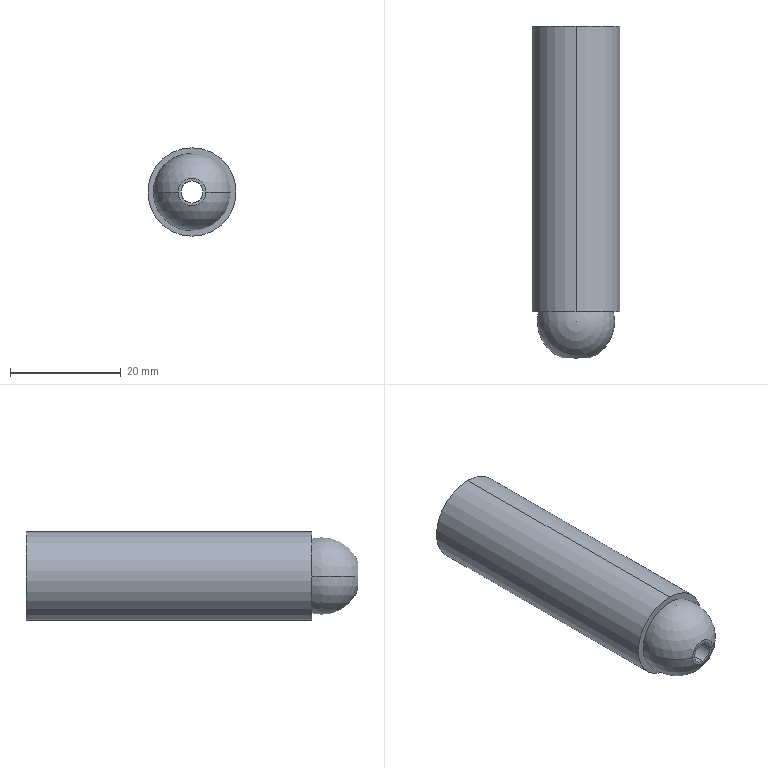Part | SolidWorks | features Revolution 1 | 1 solid | 11 faces | box 16 x 60 x 16 mm | volume 9983 mm3 | cylinder 4 | sphere 4 | plane 3 | commonest cylinder face diameters 4 x2 16 x2
STEP:
#1=CARTESIAN_POINT('',(0.,60.,-8.));
#2=VERTEX_POINT('',#1);
#3=CARTESIAN_POINT('',(0.,60.,8.));
#4=VERTEX_POINT('',#3);
#5=CARTESIAN_POINT('',(0.,60.,0.));
#6=DIRECTION('',(0.,-1.,0.));
#7=DIRECTION('',(0.,0.,-1.));
#8=AXIS2_PLACEMENT_3D('',#5,#6,#7);
#9=CIRCLE('',#8,8.);
#10=EDGE_CURVE('',#2,#4,#9,.T.);
#11=ORIENTED_EDGE('',*,*,#10,.T.);
#12=CARTESIAN_POINT('',(0.,8.392,8.));
#13=VERTEX_POINT('',#12);
#14=CARTESIAN_POINT('',(0.,0.,8.));
#15=DIRECTION('',(0.,-1.,0.));
#16=VECTOR('',#15,1000.);
#17=LINE('',#14,#16);
#18=EDGE_CURVE('',#4,#13,#17,.T.);
#19=ORIENTED_EDGE('',*,*,#18,.T.);
#20=CARTESIAN_POINT('',(0.,8.392,-8.));
#21=VERTEX_POINT('',#20);
#22=CARTESIAN_POINT('',(0.,8.392,0.));
#23=DIRECTION('',(0.,-1.,0.));
#24=DIRECTION('',(0.,0.,-1.));
#25=AXIS2_PLACEMENT_3D('',#22,#23,#24);
#26=CIRCLE('',#25,8.);
#27=EDGE_CURVE('',#21,#13,#26,.T.);
#28=ORIENTED_EDGE('',*,*,#27,.F.);
#29=CARTESIAN_POINT('',(0.,0.,-8.));
#30=DIRECTION('',(0.,-1.,0.));
#31=VECTOR('',#30,1000.);
#32=LINE('',#29,#31);
#33=EDGE_CURVE('',#2,#21,#32,.T.);
#34=ORIENTED_EDGE('',*,*,#33,.F.);
#35=EDGE_LOOP('',(#11,#19,#28,#34));
#36=FACE_OUTER_BOUND('',#35,.T.);
#37=CARTESIAN_POINT('',(0.,0.,0.));
#38=DIRECTION('',(0.,-1.,0.));
#39=DIRECTION('',(0.,0.,-1.));
#40=AXIS2_PLACEMENT_3D('',#37,#38,#39);
#41=CYLINDRICAL_SURFACE('',#40,8.);
#42=ADVANCED_FACE('',(#36),#41,.T.);
#43=CARTESIAN_POINT('',(7.,60.,0.));
#44=VERTEX_POINT('',#43);
#45=CARTESIAN_POINT('',(-7.,60.,0.));
#46=VERTEX_POINT('',#45);
#47=CARTESIAN_POINT('',(0.,60.,0.));
#48=DIRECTION('',(0.,-1.,0.));
#49=DIRECTION('',(0.,0.,-1.));
#50=AXIS2_PLACEMENT_3D('',#47,#48,#49);
#51=CIRCLE('',#50,7.);
#52=EDGE_CURVE('',#44,#46,#51,.T.);
#53=ORIENTED_EDGE('',*,*,#52,.F.);
#54=CARTESIAN_POINT('',(2.,53.292,0.));
#55=VERTEX_POINT('',#54);
#56=CARTESIAN_POINT('',(0.,60.,0.));
#57=DIRECTION('',(0.,0.,-1.));
#58=DIRECTION('',(-1.,0.,0.));
#59=AXIS2_PLACEMENT_3D('',#56,#57,#58);
#60=CIRCLE('',#59,7.);
#61=EDGE_CURVE('',#44,#55,#60,.T.);
#62=ORIENTED_EDGE('',*,*,#61,.T.);
#63=CARTESIAN_POINT('',(0.,53.292,2.));
#64=VERTEX_POINT('',#63);
#65=CARTESIAN_POINT('',(0.,53.292,0.));
#66=DIRECTION('',(0.,-1.,0.));
#67=DIRECTION('',(0.,0.,-1.));
#68=AXIS2_PLACEMENT_3D('',#65,#66,#67);
#69=CIRCLE('',#68,2.);
#70=EDGE_CURVE('',#55,#64,#69,.T.);
#71=ORIENTED_EDGE('',*,*,#70,.T.);
#72=CARTESIAN_POINT('',(-2.,53.292,0.));
#73=VERTEX_POINT('',#72);
#74=CARTESIAN_POINT('',(0.,53.292,0.));
#75=DIRECTION('',(0.,-1.,0.));
#76=DIRECTION('',(0.,0.,-1.));
#77=AXIS2_PLACEMENT_3D('',#74,#75,#76);
#78=CIRCLE('',#77,2.);
#79=EDGE_CURVE('',#64,#73,#78,.T.);
#80=ORIENTED_EDGE('',*,*,#79,.T.);
#81=CARTESIAN_POINT('',(0.,60.,0.));
#82=DIRECTION('',(0.,0.,1.));
#83=DIRECTION('',(1.,0.,0.));
#84=AXIS2_PLACEMENT_3D('',#81,#82,#83);
#85=CIRCLE('',#84,7.);
#86=EDGE_CURVE('',#46,#73,#85,.T.);
#87=ORIENTED_EDGE('',*,*,#86,.F.);
#88=EDGE_LOOP('',(#53,#62,#71,#80,#87));
#89=FACE_OUTER_BOUND('',#88,.T.);
#90=CARTESIAN_POINT('',(0.,60.,0.));
#91=DIRECTION('',(0.,0.,-1.));
#92=DIRECTION('',(-1.,0.,0.));
#93=AXIS2_PLACEMENT_3D('',#90,#91,#92);
#94=SPHERICAL_SURFACE('',#93,7.);
#95=ADVANCED_FACE('',(#89),#94,.F.);
#96=ORIENTED_EDGE('',*,*,#79,.F.);
#97=CARTESIAN_POINT('',(0.,0.,2.));
#98=VERTEX_POINT('',#97);
#99=CARTESIAN_POINT('',(0.,0.,2.));
#100=DIRECTION('',(0.,-1.,0.));
#101=VECTOR('',#100,1000.);
#102=LINE('',#99,#101);
#103=EDGE_CURVE('',#64,#98,#102,.T.);
#104=ORIENTED_EDGE('',*,*,#103,.T.);
#105=CARTESIAN_POINT('',(0.,0.,-2.));
#106=VERTEX_POINT('',#105);
#107=CARTESIAN_POINT('',(0.,0.,0.));
#108=DIRECTION('',(0.,-1.,0.));
#109=DIRECTION('',(0.,0.,-1.));
#110=AXIS2_PLACEMENT_3D('',#107,#108,#109);
#111=CIRCLE('',#110,2.);
#112=EDGE_CURVE('',#98,#106,#111,.T.);
#113=ORIENTED_EDGE('',*,*,#112,.T.);
#114=CARTESIAN_POINT('',(0.,53.292,-2.));
#115=VERTEX_POINT('',#114);
#116=CARTESIAN_POINT('',(0.,0.,-2.));
#117=DIRECTION('',(0.,-1.,0.));
#118=VECTOR('',#117,1000.);
#119=LINE('',#116,#118);
#120=EDGE_CURVE('',#115,#106,#119,.T.);
#121=ORIENTED_EDGE('',*,*,#120,.F.);
#122=CARTESIAN_POINT('',(0.,53.292,0.));
#123=DIRECTION('',(0.,-1.,0.));
#124=DIRECTION('',(0.,0.,-1.));
#125=AXIS2_PLACEMENT_3D('',#122,#123,#124);
#126=CIRCLE('',#125,2.);
#127=EDGE_CURVE('',#73,#115,#126,.T.);
#128=ORIENTED_EDGE('',*,*,#127,.F.);
#129=EDGE_LOOP('',(#96,#104,#113,#121,#128));
#130=FACE_OUTER_BOUND('',#129,.T.);
#131=CARTESIAN_POINT('',(0.,0.,0.));
#132=DIRECTION('',(0.,-1.,0.));
#133=DIRECTION('',(0.,0.,-1.));
#134=AXIS2_PLACEMENT_3D('',#131,#132,#133);
#135=CYLINDRICAL_SURFACE('',#134,2.);
#136=ADVANCED_FACE('',(#130),#135,.F.);
#137=CARTESIAN_POINT('',(-6.75,8.392,0.));
#138=VERTEX_POINT('',#137);
#139=CARTESIAN_POINT('',(6.75,8.392,0.));
#140=VERTEX_POINT('',#139);
#141=CARTESIAN_POINT('',(0.,8.392,0.));
#142=DIRECTION('',(0.,-1.,0.));
#143=DIRECTION('',(0.,0.,-1.));
#144=AXIS2_PLACEMENT_3D('',#141,#142,#143);
#145=CIRCLE('',#144,6.75);
#146=EDGE_CURVE('',#138,#140,#145,.T.);
#147=ORIENTED_EDGE('',*,*,#146,.T.);
#148=CARTESIAN_POINT('',(2.5,0.,0.));
#149=VERTEX_POINT('',#148);
#150=CARTESIAN_POINT('',(0.,6.538,0.));
#151=DIRECTION('',(0.,0.,-1.));
#152=DIRECTION('',(-1.,0.,0.));
#153=AXIS2_PLACEMENT_3D('',#150,#151,#152);
#154=CIRCLE('',#153,7.);
#155=EDGE_CURVE('',#140,#149,#154,.T.);
#156=ORIENTED_EDGE('',*,*,#155,.T.);
#157=CARTESIAN_POINT('',(-2.5,0.,0.));
#158=VERTEX_POINT('',#157);
#159=CARTESIAN_POINT('',(0.,0.,0.));
#160=DIRECTION('',(0.,-1.,0.));
#161=DIRECTION('',(0.,0.,-1.));
#162=AXIS2_PLACEMENT_3D('',#159,#160,#161);
#163=CIRCLE('',#162,2.5);
#164=EDGE_CURVE('',#158,#149,#163,.T.);
#165=ORIENTED_EDGE('',*,*,#164,.F.);
#166=CARTESIAN_POINT('',(0.,6.538,0.));
#167=DIRECTION('',(0.,0.,1.));
#168=DIRECTION('',(1.,0.,0.));
#169=AXIS2_PLACEMENT_3D('',#166,#167,#168);
#170=CIRCLE('',#169,7.);
#171=EDGE_CURVE('',#138,#158,#170,.T.);
#172=ORIENTED_EDGE('',*,*,#171,.F.);
#173=EDGE_LOOP('',(#147,#156,#165,#172));
#174=FACE_OUTER_BOUND('',#173,.T.);
#175=CARTESIAN_POINT('',(0.,6.538,0.));
#176=DIRECTION('',(0.,0.,-1.));
#177=DIRECTION('',(-1.,0.,0.));
#178=AXIS2_PLACEMENT_3D('',#175,#176,#177);
#179=SPHERICAL_SURFACE('',#178,7.);
#180=ADVANCED_FACE('',(#174),#179,.T.);
#181=ORIENTED_EDGE('',*,*,#155,.F.);
#182=CARTESIAN_POINT('',(0.,8.392,0.));
#183=DIRECTION('',(0.,-1.,0.));
#184=DIRECTION('',(0.,0.,-1.));
#185=AXIS2_PLACEMENT_3D('',#182,#183,#184);
#186=CIRCLE('',#185,6.75);
#187=EDGE_CURVE('',#140,#138,#186,.T.);
#188=ORIENTED_EDGE('',*,*,#187,.T.);
#189=ORIENTED_EDGE('',*,*,#171,.T.);
#190=CARTESIAN_POINT('',(0.,0.,0.));
#191=DIRECTION('',(0.,-1.,0.));
#192=DIRECTION('',(0.,0.,-1.));
#193=AXIS2_PLACEMENT_3D('',#190,#191,#192);
#194=CIRCLE('',#193,2.5);
#195=EDGE_CURVE('',#149,#158,#194,.T.);
#196=ORIENTED_EDGE('',*,*,#195,.F.);
#197=EDGE_LOOP('',(#181,#188,#189,#196));
#198=FACE_OUTER_BOUND('',#197,.T.);
#199=CARTESIAN_POINT('',(0.,6.538,0.));
#200=DIRECTION('',(0.,0.,-1.));
#201=DIRECTION('',(-1.,0.,0.));
#202=AXIS2_PLACEMENT_3D('',#199,#200,#201);
#203=SPHERICAL_SURFACE('',#202,7.);
#204=ADVANCED_FACE('',(#198),#203,.T.);
#205=CARTESIAN_POINT('',(0.,0.,0.));
#206=DIRECTION('',(0.,-1.,0.));
#207=DIRECTION('',(0.,0.,-1.));
#208=AXIS2_PLACEMENT_3D('',#205,#206,#207);
#209=CIRCLE('',#208,2.);
#210=EDGE_CURVE('',#106,#98,#209,.T.);
#211=ORIENTED_EDGE('',*,*,#210,.F.);
#212=ORIENTED_EDGE('',*,*,#112,.F.);
#213=EDGE_LOOP('',(#211,#212));
#214=FACE_BOUND('',#213,.T.);
#215=ORIENTED_EDGE('',*,*,#164,.T.);
#216=ORIENTED_EDGE('',*,*,#195,.T.);
#217=EDGE_LOOP('',(#215,#216));
#218=FACE_OUTER_BOUND('',#217,.T.);
#219=CARTESIAN_POINT('',(-2.,0.,0.));
#220=DIRECTION('',(0.,1.,0.));
#221=DIRECTION('',(0.,0.,1.));
#222=AXIS2_PLACEMENT_3D('',#219,#220,#221);
#223=PLANE('',#222);
#224=ADVANCED_FACE('',(#214,#218),#223,.F.);
#225=ORIENTED_EDGE('',*,*,#103,.F.);
#226=ORIENTED_EDGE('',*,*,#70,.F.);
#227=CARTESIAN_POINT('',(0.,53.292,0.));
#228=DIRECTION('',(0.,-1.,0.));
#229=DIRECTION('',(0.,0.,-1.));
#230=AXIS2_PLACEMENT_3D('',#227,#228,#229);
#231=CIRCLE('',#230,2.);
#232=EDGE_CURVE('',#115,#55,#231,.T.);
#233=ORIENTED_EDGE('',*,*,#232,.F.);
#234=ORIENTED_EDGE('',*,*,#120,.T.);
#235=ORIENTED_EDGE('',*,*,#210,.T.);
#236=EDGE_LOOP('',(#225,#226,#233,#234,#235));
#237=FACE_OUTER_BOUND('',#236,.T.);
#238=CARTESIAN_POINT('',(0.,0.,0.));
#239=DIRECTION('',(0.,-1.,0.));
#240=DIRECTION('',(0.,0.,-1.));
#241=AXIS2_PLACEMENT_3D('',#238,#239,#240);
#242=CYLINDRICAL_SURFACE('',#241,2.);
#243=ADVANCED_FACE('',(#237),#242,.F.);
#244=ORIENTED_EDGE('',*,*,#61,.F.);
#245=CARTESIAN_POINT('',(0.,60.,0.));
#246=DIRECTION('',(0.,-1.,0.));
#247=DIRECTION('',(0.,0.,-1.));
#248=AXIS2_PLACEMENT_3D('',#245,#246,#247);
#249=CIRCLE('',#248,7.);
#250=EDGE_CURVE('',#46,#44,#249,.T.);
#251=ORIENTED_EDGE('',*,*,#250,.F.);
#252=ORIENTED_EDGE('',*,*,#86,.T.);
#253=ORIENTED_EDGE('',*,*,#127,.T.);
#254=ORIENTED_EDGE('',*,*,#232,.T.);
#255=EDGE_LOOP('',(#244,#251,#252,#253,#254));
#256=FACE_OUTER_BOUND('',#255,.T.);
#257=CARTESIAN_POINT('',(0.,60.,0.));
#258=DIRECTION('',(0.,0.,-1.));
#259=DIRECTION('',(-1.,0.,0.));
#260=AXIS2_PLACEMENT_3D('',#257,#258,#259);
#261=SPHERICAL_SURFACE('',#260,7.);
#262=ADVANCED_FACE('',(#256),#261,.F.);
#263=ORIENTED_EDGE('',*,*,#10,.F.);
#264=CARTESIAN_POINT('',(0.,60.,0.));
#265=DIRECTION('',(0.,-1.,0.));
#266=DIRECTION('',(0.,0.,-1.));
#267=AXIS2_PLACEMENT_3D('',#264,#265,#266);
#268=CIRCLE('',#267,8.);
#269=EDGE_CURVE('',#4,#2,#268,.T.);
#270=ORIENTED_EDGE('',*,*,#269,.F.);
#271=EDGE_LOOP('',(#263,#270));
#272=FACE_OUTER_BOUND('',#271,.T.);
#273=ORIENTED_EDGE('',*,*,#250,.T.);
#274=ORIENTED_EDGE('',*,*,#52,.T.);
#275=EDGE_LOOP('',(#273,#274));
#276=FACE_BOUND('',#275,.T.);
#277=CARTESIAN_POINT('',(-7.,60.,0.));
#278=DIRECTION('',(0.,-1.,0.));
#279=DIRECTION('',(0.,0.,-1.));
#280=AXIS2_PLACEMENT_3D('',#277,#278,#279);
#281=PLANE('',#280);
#282=ADVANCED_FACE('',(#272,#276),#281,.F.);
#283=ORIENTED_EDGE('',*,*,#18,.F.);
#284=ORIENTED_EDGE('',*,*,#269,.T.);
#285=ORIENTED_EDGE('',*,*,#33,.T.);
#286=CARTESIAN_POINT('',(0.,8.392,0.));
#287=DIRECTION('',(0.,-1.,0.));
#288=DIRECTION('',(0.,0.,-1.));
#289=AXIS2_PLACEMENT_3D('',#286,#287,#288);
#290=CIRCLE('',#289,8.);
#291=EDGE_CURVE('',#13,#21,#290,.T.);
#292=ORIENTED_EDGE('',*,*,#291,.F.);
#293=EDGE_LOOP('',(#283,#284,#285,#292));
#294=FACE_OUTER_BOUND('',#293,.T.);
#295=CARTESIAN_POINT('',(0.,0.,0.));
#296=DIRECTION('',(0.,-1.,0.));
#297=DIRECTION('',(0.,0.,-1.));
#298=AXIS2_PLACEMENT_3D('',#295,#296,#297);
#299=CYLINDRICAL_SURFACE('',#298,8.);
#300=ADVANCED_FACE('',(#294),#299,.T.);
#301=ORIENTED_EDGE('',*,*,#146,.F.);
#302=ORIENTED_EDGE('',*,*,#187,.F.);
#303=EDGE_LOOP('',(#301,#302));
#304=FACE_BOUND('',#303,.T.);
#305=ORIENTED_EDGE('',*,*,#27,.T.);
#306=ORIENTED_EDGE('',*,*,#291,.T.);
#307=EDGE_LOOP('',(#305,#306));
#308=FACE_OUTER_BOUND('',#307,.T.);
#309=CARTESIAN_POINT('',(-8.,8.392,0.));
#310=DIRECTION('',(0.,1.,0.));
#311=DIRECTION('',(0.,0.,1.));
#312=AXIS2_PLACEMENT_3D('',#309,#310,#311);
#313=PLANE('',#312);
#314=ADVANCED_FACE('',(#304,#308),#313,.F.);
#315=CLOSED_SHELL('',(#42,#95,#136,#180,#204,#224,#243,#262,#282,#300,#314));
#316=MANIFOLD_SOLID_BREP('',#315);
#317=CARTESIAN_POINT('',(0.,0.,0.));
#318=DIRECTION('',(0.,0.,1.));
#319=DIRECTION('',(1.,0.,0.));
#320=AXIS2_PLACEMENT_3D('',#317,#318,#319);
#321=(LENGTH_UNIT()NAMED_UNIT(*)SI_UNIT(.MILLI.,.METRE.));
#322=UNCERTAINTY_MEASURE_WITH_UNIT(LENGTH_MEASURE(0.00001),#321,'','');
#323=(NAMED_UNIT(*)PLANE_ANGLE_UNIT()SI_UNIT($,.RADIAN.));
#324=(NAMED_UNIT(*)SI_UNIT($,.STERADIAN.)SOLID_ANGLE_UNIT());
#325=(GEOMETRIC_REPRESENTATION_CONTEXT(3)GLOBAL_UNCERTAINTY_ASSIGNED_CONTEXT((#322))GLOBAL_UNIT_ASSIGNED_CONTEXT((#321,#323,#324))REPRESENTATION_CONTEXT('',''));
#326=ADVANCED_BREP_SHAPE_REPRESENTATION('',(#316,#320),#325);